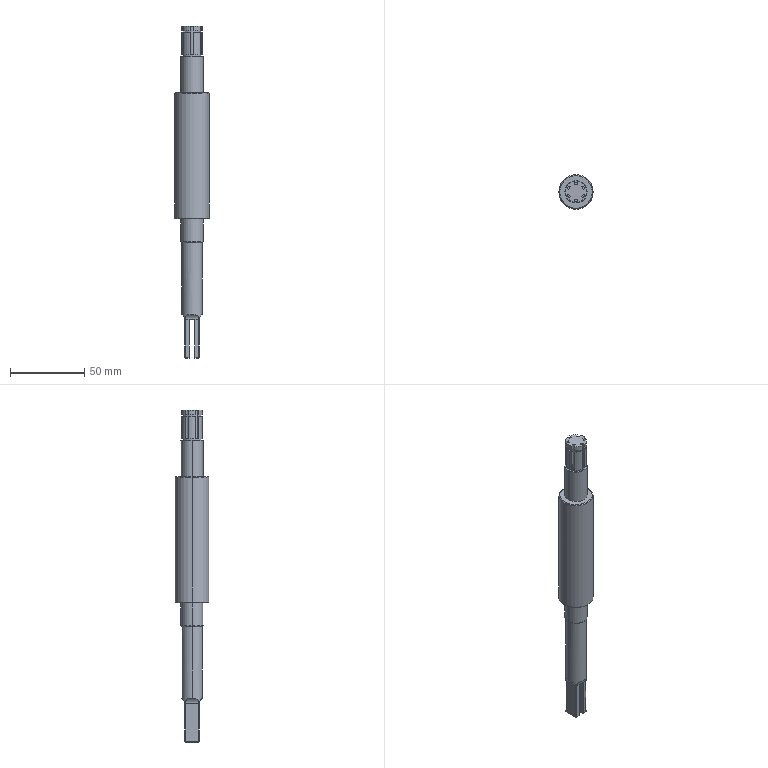Part | STEP file | Driven drive shaft (spline) SGN-5-06 | 1 solid | 120 faces | box 23 x 23 x 223.85 mm | volume 54404 mm3 | cylinder 53 | plane 51 | cone 8 | spline 4 | sphere 4 | commonest cylinder face diameters 14 x16 1 x10 12.8 x9 10.002 x6 8 x4 15 x4